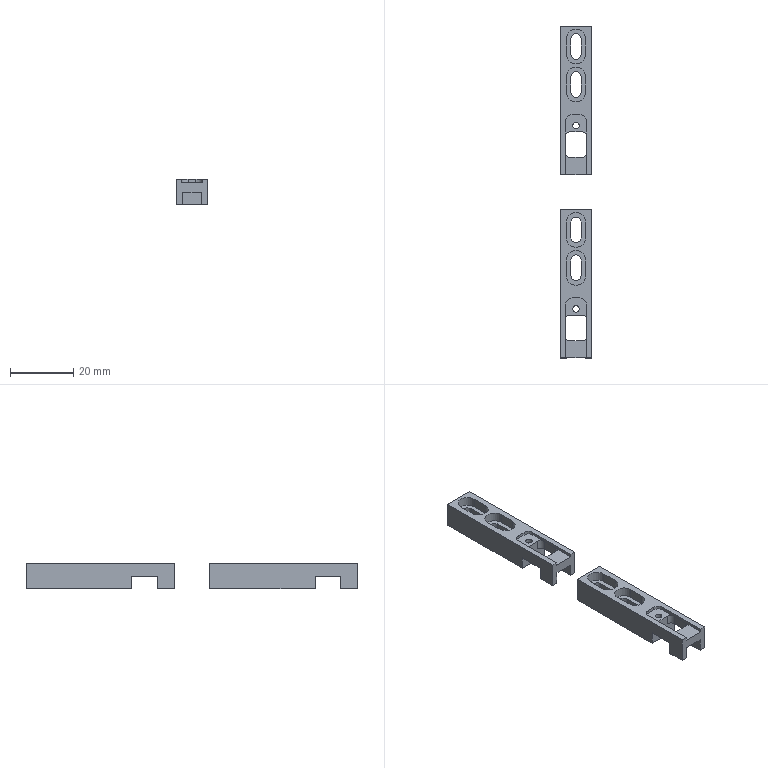Part | 2 solids | 98 faces | box 10 x 105 x 8 mm | volume 4822 mm3 | plane 68 | cylinder 30 | commonest cylinder face diameters 3 x8 3.2 x8 6 x8 4 x4 2.05 x2